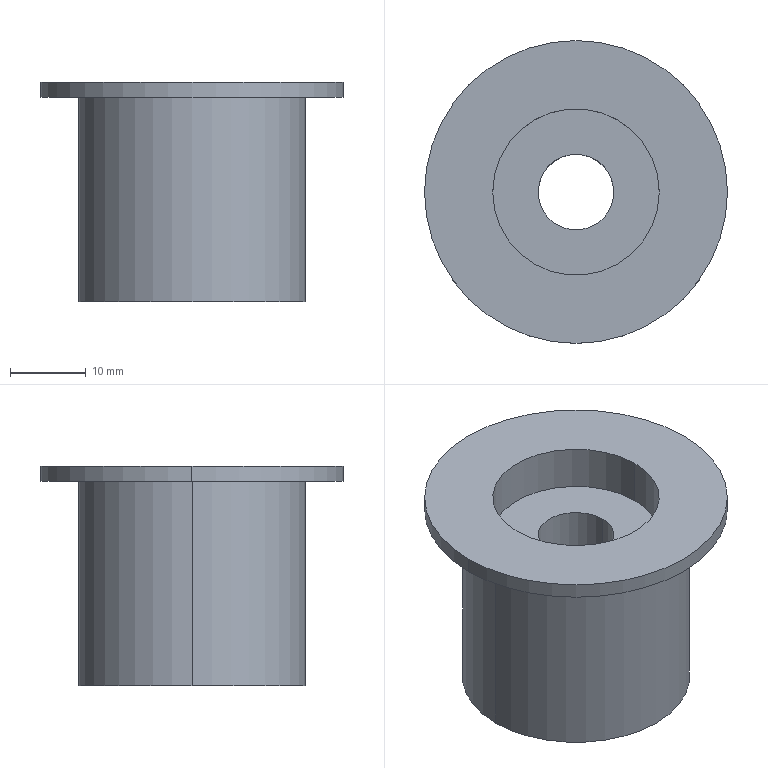Part | STEP file | Tensioning pulley QY-1-12 | 1 solid | 15 faces | box 40 x 40 x 29 mm | volume 15702 mm3 | cylinder 10 | plane 5 | commonest cylinder face diameters 22 x4 10 x2 30 x2 40 x2
STEP:
#1=CARTESIAN_POINT('',(0.,0.,0.));
#2=DIRECTION('',(0.,0.,1.));
#3=DIRECTION('',(1.,0.,0.));
#4=AXIS2_PLACEMENT_3D('',#1,#2,#3);
#5=CARTESIAN_POINT('',(20.,0.,12.5));
#6=VERTEX_POINT('',#5);
#7=CARTESIAN_POINT('',(-20.,0.,12.5));
#8=VERTEX_POINT('',#7);
#9=CARTESIAN_POINT('',(0.,0.,12.5));
#10=DIRECTION('',(0.,0.,1.));
#11=DIRECTION('',(1.,0.,0.));
#12=AXIS2_PLACEMENT_3D('',#9,#10,#11);
#13=CIRCLE('',#12,20.);
#14=CARTESIAN_POINT('',(0.,0.,12.5));
#15=DIRECTION('',(0.,0.,1.));
#16=DIRECTION('',(1.,0.,0.));
#17=AXIS2_PLACEMENT_3D('',#14,#15,#16);
#18=CYLINDRICAL_SURFACE('',#17,20.);
#19=CARTESIAN_POINT('',(0.,0.));
#20=DIRECTION('',(1.,0.));
#21=VECTOR('',#20,1.);
#22=LINE('',#19,#21);
#23=(GEOMETRIC_REPRESENTATION_CONTEXT(2)PARAMETRIC_REPRESENTATION_CONTEXT()REPRESENTATION_CONTEXT('',''));
#24=DEFINITIONAL_REPRESENTATION('',(#22),#23);
#25=PCURVE('',#18,#24);
#26=CARTESIAN_POINT('',(0.,0.,12.5));
#27=DIRECTION('',(0.,0.,1.));
#28=DIRECTION('',(1.,0.,0.));
#29=AXIS2_PLACEMENT_3D('',#26,#27,#28);
#30=PLANE('',#29);
#31=CARTESIAN_POINT('',(0.,0.));
#32=DIRECTION('',(1.,0.));
#33=AXIS2_PLACEMENT_2D('',#31,#32);
#34=CIRCLE('',#33,20.);
#35=(GEOMETRIC_REPRESENTATION_CONTEXT(2)PARAMETRIC_REPRESENTATION_CONTEXT()REPRESENTATION_CONTEXT('',''));
#36=DEFINITIONAL_REPRESENTATION('',(#34),#35);
#37=PCURVE('',#30,#36);
#38=SURFACE_CURVE('',#13,(#25,#37),.PCURVE_S1.);
#39=EDGE_CURVE('',#6,#8,#38,.T.);
#40=ORIENTED_EDGE('',*,*,#39,.T.);
#41=CARTESIAN_POINT('',(-20.,0.,14.5));
#42=VERTEX_POINT('',#41);
#43=CARTESIAN_POINT('',(-20.,0.,12.5));
#44=DIRECTION('',(0.,0.,1.));
#45=VECTOR('',#44,1.);
#46=LINE('',#43,#45);
#47=CARTESIAN_POINT('',(3.142,0.));
#48=DIRECTION('',(0.,1.));
#49=VECTOR('',#48,1.);
#50=LINE('',#47,#49);
#51=(GEOMETRIC_REPRESENTATION_CONTEXT(2)PARAMETRIC_REPRESENTATION_CONTEXT()REPRESENTATION_CONTEXT('',''));
#52=DEFINITIONAL_REPRESENTATION('',(#50),#51);
#53=PCURVE('',#18,#52);
#54=CARTESIAN_POINT('',(0.,0.,12.5));
#55=DIRECTION('',(0.,0.,1.));
#56=DIRECTION('',(1.,0.,0.));
#57=AXIS2_PLACEMENT_3D('',#54,#55,#56);
#58=CYLINDRICAL_SURFACE('',#57,20.);
#59=CARTESIAN_POINT('',(3.142,0.));
#60=DIRECTION('',(0.,1.));
#61=VECTOR('',#60,1.);
#62=LINE('',#59,#61);
#63=(GEOMETRIC_REPRESENTATION_CONTEXT(2)PARAMETRIC_REPRESENTATION_CONTEXT()REPRESENTATION_CONTEXT('',''));
#64=DEFINITIONAL_REPRESENTATION('',(#62),#63);
#65=PCURVE('',#58,#64);
#66=SURFACE_CURVE('',#46,(#53,#65),.PCURVE_S1.);
#67=EDGE_CURVE('',#8,#42,#66,.T.);
#68=ORIENTED_EDGE('',*,*,#67,.T.);
#69=CARTESIAN_POINT('',(20.,0.,14.5));
#70=VERTEX_POINT('',#69);
#71=CARTESIAN_POINT('',(0.,0.,14.5));
#72=DIRECTION('',(0.,0.,1.));
#73=DIRECTION('',(1.,0.,0.));
#74=AXIS2_PLACEMENT_3D('',#71,#72,#73);
#75=CIRCLE('',#74,20.);
#76=CARTESIAN_POINT('',(0.,2.));
#77=DIRECTION('',(1.,0.));
#78=VECTOR('',#77,1.);
#79=LINE('',#76,#78);
#80=(GEOMETRIC_REPRESENTATION_CONTEXT(2)PARAMETRIC_REPRESENTATION_CONTEXT()REPRESENTATION_CONTEXT('',''));
#81=DEFINITIONAL_REPRESENTATION('',(#79),#80);
#82=PCURVE('',#18,#81);
#83=CARTESIAN_POINT('',(0.,0.,14.5));
#84=DIRECTION('',(0.,0.,1.));
#85=DIRECTION('',(1.,0.,0.));
#86=AXIS2_PLACEMENT_3D('',#83,#84,#85);
#87=PLANE('',#86);
#88=CARTESIAN_POINT('',(0.,0.));
#89=DIRECTION('',(1.,0.));
#90=AXIS2_PLACEMENT_2D('',#88,#89);
#91=CIRCLE('',#90,20.);
#92=(GEOMETRIC_REPRESENTATION_CONTEXT(2)PARAMETRIC_REPRESENTATION_CONTEXT()REPRESENTATION_CONTEXT('',''));
#93=DEFINITIONAL_REPRESENTATION('',(#91),#92);
#94=PCURVE('',#87,#93);
#95=SURFACE_CURVE('',#75,(#82,#94),.PCURVE_S1.);
#96=EDGE_CURVE('',#70,#42,#95,.T.);
#97=ORIENTED_EDGE('',*,*,#96,.F.);
#98=CARTESIAN_POINT('',(20.,0.,12.5));
#99=DIRECTION('',(0.,0.,1.));
#100=VECTOR('',#99,1.);
#101=LINE('',#98,#100);
#102=CARTESIAN_POINT('',(0.,0.));
#103=DIRECTION('',(0.,1.));
#104=VECTOR('',#103,1.);
#105=LINE('',#102,#104);
#106=(GEOMETRIC_REPRESENTATION_CONTEXT(2)PARAMETRIC_REPRESENTATION_CONTEXT()REPRESENTATION_CONTEXT('',''));
#107=DEFINITIONAL_REPRESENTATION('',(#105),#106);
#108=PCURVE('',#18,#107);
#109=CARTESIAN_POINT('',(6.283,0.));
#110=DIRECTION('',(0.,1.));
#111=VECTOR('',#110,1.);
#112=LINE('',#109,#111);
#113=(GEOMETRIC_REPRESENTATION_CONTEXT(2)PARAMETRIC_REPRESENTATION_CONTEXT()REPRESENTATION_CONTEXT('',''));
#114=DEFINITIONAL_REPRESENTATION('',(#112),#113);
#115=PCURVE('',#58,#114);
#116=SURFACE_CURVE('',#101,(#108,#115),.PCURVE_S1.);
#117=EDGE_CURVE('',#6,#70,#116,.T.);
#118=ORIENTED_EDGE('',*,*,#117,.F.);
#119=EDGE_LOOP('',(#40,#68,#97,#118));
#120=FACE_BOUND('',#119,.T.);
#121=ADVANCED_FACE('',(#120),#18,.T.);
#122=CARTESIAN_POINT('',(-5.,0.,8.5));
#123=VERTEX_POINT('',#122);
#124=CARTESIAN_POINT('',(-5.,0.,-8.5));
#125=VERTEX_POINT('',#124);
#126=CARTESIAN_POINT('',(-5.,0.,8.5));
#127=DIRECTION('',(0.,0.,-1.));
#128=VECTOR('',#127,1.);
#129=LINE('',#126,#128);
#130=CARTESIAN_POINT('',(0.,0.,8.5));
#131=DIRECTION('',(0.,0.,-1.));
#132=DIRECTION('',(-1.,0.,0.));
#133=AXIS2_PLACEMENT_3D('',#130,#131,#132);
#134=CYLINDRICAL_SURFACE('',#133,5.);
#135=CARTESIAN_POINT('',(6.283,0.));
#136=DIRECTION('',(0.,1.));
#137=VECTOR('',#136,1.);
#138=LINE('',#135,#137);
#139=(GEOMETRIC_REPRESENTATION_CONTEXT(2)PARAMETRIC_REPRESENTATION_CONTEXT()REPRESENTATION_CONTEXT('',''));
#140=DEFINITIONAL_REPRESENTATION('',(#138),#139);
#141=PCURVE('',#134,#140);
#142=CARTESIAN_POINT('',(0.,0.,8.5));
#143=DIRECTION('',(0.,0.,-1.));
#144=DIRECTION('',(-1.,0.,0.));
#145=AXIS2_PLACEMENT_3D('',#142,#143,#144);
#146=CYLINDRICAL_SURFACE('',#145,5.);
#147=CARTESIAN_POINT('',(0.,0.));
#148=DIRECTION('',(0.,1.));
#149=VECTOR('',#148,1.);
#150=LINE('',#147,#149);
#151=(GEOMETRIC_REPRESENTATION_CONTEXT(2)PARAMETRIC_REPRESENTATION_CONTEXT()REPRESENTATION_CONTEXT('',''));
#152=DEFINITIONAL_REPRESENTATION('',(#150),#151);
#153=PCURVE('',#146,#152);
#154=SURFACE_CURVE('',#129,(#141,#153),.PCURVE_S1.);
#155=EDGE_CURVE('',#123,#125,#154,.T.);
#156=ORIENTED_EDGE('',*,*,#155,.T.);
#157=CARTESIAN_POINT('',(5.,0.,-8.5));
#158=VERTEX_POINT('',#157);
#159=CARTESIAN_POINT('',(0.,0.,-8.5));
#160=DIRECTION('',(0.,0.,1.));
#161=DIRECTION('',(1.,0.,0.));
#162=AXIS2_PLACEMENT_3D('',#159,#160,#161);
#163=CIRCLE('',#162,5.);
#164=CARTESIAN_POINT('',(9.425,17.));
#165=DIRECTION('',(-1.,0.));
#166=VECTOR('',#165,1.);
#167=LINE('',#164,#166);
#168=(GEOMETRIC_REPRESENTATION_CONTEXT(2)PARAMETRIC_REPRESENTATION_CONTEXT()REPRESENTATION_CONTEXT('',''));
#169=DEFINITIONAL_REPRESENTATION('',(#167),#168);
#170=PCURVE('',#134,#169);
#171=CARTESIAN_POINT('',(0.,0.,-8.5));
#172=DIRECTION('',(0.,0.,1.));
#173=DIRECTION('',(1.,0.,0.));
#174=AXIS2_PLACEMENT_3D('',#171,#172,#173);
#175=PLANE('',#174);
#176=CARTESIAN_POINT('',(0.,0.));
#177=DIRECTION('',(1.,0.));
#178=AXIS2_PLACEMENT_2D('',#176,#177);
#179=CIRCLE('',#178,5.);
#180=(GEOMETRIC_REPRESENTATION_CONTEXT(2)PARAMETRIC_REPRESENTATION_CONTEXT()REPRESENTATION_CONTEXT('',''));
#181=DEFINITIONAL_REPRESENTATION('',(#179),#180);
#182=PCURVE('',#175,#181);
#183=SURFACE_CURVE('',#163,(#170,#182),.PCURVE_S1.);
#184=EDGE_CURVE('',#125,#158,#183,.T.);
#185=ORIENTED_EDGE('',*,*,#184,.T.);
#186=CARTESIAN_POINT('',(5.,0.,8.5));
#187=VERTEX_POINT('',#186);
#188=CARTESIAN_POINT('',(5.,0.,8.5));
#189=DIRECTION('',(0.,0.,-1.));
#190=VECTOR('',#189,1.);
#191=LINE('',#188,#190);
#192=CARTESIAN_POINT('',(3.142,0.));
#193=DIRECTION('',(0.,1.));
#194=VECTOR('',#193,1.);
#195=LINE('',#192,#194);
#196=(GEOMETRIC_REPRESENTATION_CONTEXT(2)PARAMETRIC_REPRESENTATION_CONTEXT()REPRESENTATION_CONTEXT('',''));
#197=DEFINITIONAL_REPRESENTATION('',(#195),#196);
#198=PCURVE('',#134,#197);
#199=CARTESIAN_POINT('',(3.142,0.));
#200=DIRECTION('',(0.,1.));
#201=VECTOR('',#200,1.);
#202=LINE('',#199,#201);
#203=(GEOMETRIC_REPRESENTATION_CONTEXT(2)PARAMETRIC_REPRESENTATION_CONTEXT()REPRESENTATION_CONTEXT('',''));
#204=DEFINITIONAL_REPRESENTATION('',(#202),#203);
#205=PCURVE('',#146,#204);
#206=SURFACE_CURVE('',#191,(#198,#205),.PCURVE_S1.);
#207=EDGE_CURVE('',#187,#158,#206,.T.);
#208=ORIENTED_EDGE('',*,*,#207,.F.);
#209=CARTESIAN_POINT('',(0.,0.,8.5));
#210=DIRECTION('',(0.,0.,1.));
#211=DIRECTION('',(1.,0.,0.));
#212=AXIS2_PLACEMENT_3D('',#209,#210,#211);
#213=CIRCLE('',#212,5.);
#214=CARTESIAN_POINT('',(9.425,0.));
#215=DIRECTION('',(-1.,0.));
#216=VECTOR('',#215,1.);
#217=LINE('',#214,#216);
#218=(GEOMETRIC_REPRESENTATION_CONTEXT(2)PARAMETRIC_REPRESENTATION_CONTEXT()REPRESENTATION_CONTEXT('',''));
#219=DEFINITIONAL_REPRESENTATION('',(#217),#218);
#220=PCURVE('',#134,#219);
#221=CARTESIAN_POINT('',(0.,0.,8.5));
#222=DIRECTION('',(0.,0.,1.));
#223=DIRECTION('',(1.,0.,0.));
#224=AXIS2_PLACEMENT_3D('',#221,#222,#223);
#225=PLANE('',#224);
#226=CARTESIAN_POINT('',(0.,0.));
#227=DIRECTION('',(1.,0.));
#228=AXIS2_PLACEMENT_2D('',#226,#227);
#229=CIRCLE('',#228,5.);
#230=(GEOMETRIC_REPRESENTATION_CONTEXT(2)PARAMETRIC_REPRESENTATION_CONTEXT()REPRESENTATION_CONTEXT('',''));
#231=DEFINITIONAL_REPRESENTATION('',(#229),#230);
#232=PCURVE('',#225,#231);
#233=SURFACE_CURVE('',#213,(#220,#232),.PCURVE_S1.);
#234=EDGE_CURVE('',#123,#187,#233,.T.);
#235=ORIENTED_EDGE('',*,*,#234,.F.);
#236=EDGE_LOOP('',(#156,#185,#208,#235));
#237=FACE_BOUND('',#236,.F.);
#238=ADVANCED_FACE('',(#237),#134,.F.);
#239=CARTESIAN_POINT('',(-11.,0.,14.5));
#240=VERTEX_POINT('',#239);
#241=CARTESIAN_POINT('',(-11.,0.,8.5));
#242=VERTEX_POINT('',#241);
#243=CARTESIAN_POINT('',(-11.,0.,14.5));
#244=DIRECTION('',(0.,0.,-1.));
#245=VECTOR('',#244,1.);
#246=LINE('',#243,#245);
#247=CARTESIAN_POINT('',(0.,0.,14.5));
#248=DIRECTION('',(0.,0.,-1.));
#249=DIRECTION('',(-1.,0.,0.));
#250=AXIS2_PLACEMENT_3D('',#247,#248,#249);
#251=CYLINDRICAL_SURFACE('',#250,11.);
#252=CARTESIAN_POINT('',(6.283,0.));
#253=DIRECTION('',(0.,1.));
#254=VECTOR('',#253,1.);
#255=LINE('',#252,#254);
#256=(GEOMETRIC_REPRESENTATION_CONTEXT(2)PARAMETRIC_REPRESENTATION_CONTEXT()REPRESENTATION_CONTEXT('',''));
#257=DEFINITIONAL_REPRESENTATION('',(#255),#256);
#258=PCURVE('',#251,#257);
#259=CARTESIAN_POINT('',(0.,0.,14.5));
#260=DIRECTION('',(0.,0.,-1.));
#261=DIRECTION('',(-1.,0.,0.));
#262=AXIS2_PLACEMENT_3D('',#259,#260,#261);
#263=CYLINDRICAL_SURFACE('',#262,11.);
#264=CARTESIAN_POINT('',(0.,0.));
#265=DIRECTION('',(0.,1.));
#266=VECTOR('',#265,1.);
#267=LINE('',#264,#266);
#268=(GEOMETRIC_REPRESENTATION_CONTEXT(2)PARAMETRIC_REPRESENTATION_CONTEXT()REPRESENTATION_CONTEXT('',''));
#269=DEFINITIONAL_REPRESENTATION('',(#267),#268);
#270=PCURVE('',#263,#269);
#271=SURFACE_CURVE('',#246,(#258,#270),.PCURVE_S1.);
#272=EDGE_CURVE('',#240,#242,#271,.T.);
#273=ORIENTED_EDGE('',*,*,#272,.T.);
#274=CARTESIAN_POINT('',(11.,0.,8.5));
#275=VERTEX_POINT('',#274);
#276=CARTESIAN_POINT('',(0.,0.,8.5));
#277=DIRECTION('',(0.,0.,1.));
#278=DIRECTION('',(1.,0.,0.));
#279=AXIS2_PLACEMENT_3D('',#276,#277,#278);
#280=CIRCLE('',#279,11.);
#281=CARTESIAN_POINT('',(9.425,6.));
#282=DIRECTION('',(-1.,0.));
#283=VECTOR('',#282,1.);
#284=LINE('',#281,#283);
#285=(GEOMETRIC_REPRESENTATION_CONTEXT(2)PARAMETRIC_REPRESENTATION_CONTEXT()REPRESENTATION_CONTEXT('',''));
#286=DEFINITIONAL_REPRESENTATION('',(#284),#285);
#287=PCURVE('',#251,#286);
#288=CARTESIAN_POINT('',(0.,0.));
#289=DIRECTION('',(1.,0.));
#290=AXIS2_PLACEMENT_2D('',#288,#289);
#291=CIRCLE('',#290,11.);
#292=(GEOMETRIC_REPRESENTATION_CONTEXT(2)PARAMETRIC_REPRESENTATION_CONTEXT()REPRESENTATION_CONTEXT('',''));
#293=DEFINITIONAL_REPRESENTATION('',(#291),#292);
#294=PCURVE('',#225,#293);
#295=SURFACE_CURVE('',#280,(#287,#294),.PCURVE_S1.);
#296=EDGE_CURVE('',#242,#275,#295,.T.);
#297=ORIENTED_EDGE('',*,*,#296,.T.);
#298=CARTESIAN_POINT('',(11.,0.,14.5));
#299=VERTEX_POINT('',#298);
#300=CARTESIAN_POINT('',(11.,0.,14.5));
#301=DIRECTION('',(0.,0.,-1.));
#302=VECTOR('',#301,1.);
#303=LINE('',#300,#302);
#304=CARTESIAN_POINT('',(3.142,0.));
#305=DIRECTION('',(0.,1.));
#306=VECTOR('',#305,1.);
#307=LINE('',#304,#306);
#308=(GEOMETRIC_REPRESENTATION_CONTEXT(2)PARAMETRIC_REPRESENTATION_CONTEXT()REPRESENTATION_CONTEXT('',''));
#309=DEFINITIONAL_REPRESENTATION('',(#307),#308);
#310=PCURVE('',#251,#309);
#311=CARTESIAN_POINT('',(3.142,0.));
#312=DIRECTION('',(0.,1.));
#313=VECTOR('',#312,1.);
#314=LINE('',#311,#313);
#315=(GEOMETRIC_REPRESENTATION_CONTEXT(2)PARAMETRIC_REPRESENTATION_CONTEXT()REPRESENTATION_CONTEXT('',''));
#316=DEFINITIONAL_REPRESENTATION('',(#314),#315);
#317=PCURVE('',#263,#316);
#318=SURFACE_CURVE('',#303,(#310,#317),.PCURVE_S1.);
#319=EDGE_CURVE('',#299,#275,#318,.T.);
#320=ORIENTED_EDGE('',*,*,#319,.F.);
#321=CARTESIAN_POINT('',(0.,0.,14.5));
#322=DIRECTION('',(0.,0.,1.));
#323=DIRECTION('',(1.,0.,0.));
#324=AXIS2_PLACEMENT_3D('',#321,#322,#323);
#325=CIRCLE('',#324,11.);
#326=CARTESIAN_POINT('',(9.425,0.));
#327=DIRECTION('',(-1.,0.));
#328=VECTOR('',#327,1.);
#329=LINE('',#326,#328);
#330=(GEOMETRIC_REPRESENTATION_CONTEXT(2)PARAMETRIC_REPRESENTATION_CONTEXT()REPRESENTATION_CONTEXT('',''));
#331=DEFINITIONAL_REPRESENTATION('',(#329),#330);
#332=PCURVE('',#251,#331);
#333=CARTESIAN_POINT('',(0.,0.));
#334=DIRECTION('',(1.,0.));
#335=AXIS2_PLACEMENT_2D('',#333,#334);
#336=CIRCLE('',#335,11.);
#337=(GEOMETRIC_REPRESENTATION_CONTEXT(2)PARAMETRIC_REPRESENTATION_CONTEXT()REPRESENTATION_CONTEXT('',''));
#338=DEFINITIONAL_REPRESENTATION('',(#336),#337);
#339=PCURVE('',#87,#338);
#340=SURFACE_CURVE('',#325,(#332,#339),.PCURVE_S1.);
#341=EDGE_CURVE('',#240,#299,#340,.T.);
#342=ORIENTED_EDGE('',*,*,#341,.F.);
#343=EDGE_LOOP('',(#273,#297,#320,#342));
#344=FACE_BOUND('',#343,.F.);
#345=ADVANCED_FACE('',(#344),#251,.F.);
#346=CARTESIAN_POINT('',(-11.,0.,-8.5));
#347=VERTEX_POINT('',#346);
#348=CARTESIAN_POINT('',(-11.,0.,-14.5));
#349=VERTEX_POINT('',#348);
#350=CARTESIAN_POINT('',(-11.,0.,14.5));
#351=DIRECTION('',(0.,0.,-1.));
#352=VECTOR('',#351,1.);
#353=LINE('',#350,#352);
#354=CARTESIAN_POINT('',(0.,0.,14.5));
#355=DIRECTION('',(0.,0.,-1.));
#356=DIRECTION('',(-1.,0.,0.));
#357=AXIS2_PLACEMENT_3D('',#354,#355,#356);
#358=CYLINDRICAL_SURFACE('',#357,11.);
#359=CARTESIAN_POINT('',(6.283,0.));
#360=DIRECTION('',(0.,1.));
#361=VECTOR('',#360,1.);
#362=LINE('',#359,#361);
#363=(GEOMETRIC_REPRESENTATION_CONTEXT(2)PARAMETRIC_REPRESENTATION_CONTEXT()REPRESENTATION_CONTEXT('',''));
#364=DEFINITIONAL_REPRESENTATION('',(#362),#363);
#365=PCURVE('',#358,#364);
#366=CARTESIAN_POINT('',(0.,0.,14.5));
#367=DIRECTION('',(0.,0.,-1.));
#368=DIRECTION('',(-1.,0.,0.));
#369=AXIS2_PLACEMENT_3D('',#366,#367,#368);
#370=CYLINDRICAL_SURFACE('',#369,11.);
#371=CARTESIAN_POINT('',(0.,0.));
#372=DIRECTION('',(0.,1.));
#373=VECTOR('',#372,1.);
#374=LINE('',#371,#373);
#375=(GEOMETRIC_REPRESENTATION_CONTEXT(2)PARAMETRIC_REPRESENTATION_CONTEXT()REPRESENTATION_CONTEXT('',''));
#376=DEFINITIONAL_REPRESENTATION('',(#374),#375);
#377=PCURVE('',#370,#376);
#378=SURFACE_CURVE('',#353,(#365,#377),.PCURVE_S1.);
#379=EDGE_CURVE('',#347,#349,#378,.T.);
#380=ORIENTED_EDGE('',*,*,#379,.T.);
#381=CARTESIAN_POINT('',(11.,0.,-14.5));
#382=VERTEX_POINT('',#381);
#383=CARTESIAN_POINT('',(0.,0.,-14.5));
#384=DIRECTION('',(0.,0.,1.));
#385=DIRECTION('',(1.,0.,0.));
#386=AXIS2_PLACEMENT_3D('',#383,#384,#385);
#387=CIRCLE('',#386,11.);
#388=CARTESIAN_POINT('',(9.425,29.));
#389=DIRECTION('',(-1.,0.));
#390=VECTOR('',#389,1.);
#391=LINE('',#388,#390);
#392=(GEOMETRIC_REPRESENTATION_CONTEXT(2)PARAMETRIC_REPRESENTATION_CONTEXT()REPRESENTATION_CONTEXT('',''));
#393=DEFINITIONAL_REPRESENTATION('',(#391),#392);
#394=PCURVE('',#358,#393);
#395=CARTESIAN_POINT('',(0.,0.,-14.5));
#396=DIRECTION('',(0.,0.,1.));
#397=DIRECTION('',(1.,0.,0.));
#398=AXIS2_PLACEMENT_3D('',#395,#396,#397);
#399=PLANE('',#398);
#400=CARTESIAN_POINT('',(0.,0.));
#401=DIRECTION('',(1.,0.));
#402=AXIS2_PLACEMENT_2D('',#400,#401);
#403=CIRCLE('',#402,11.);
#404=(GEOMETRIC_REPRESENTATION_CONTEXT(2)PARAMETRIC_REPRESENTATION_CONTEXT()REPRESENTATION_CONTEXT('',''));
#405=DEFINITIONAL_REPRESENTATION('',(#403),#404);
#406=PCURVE('',#399,#405);
#407=SURFACE_CURVE('',#387,(#394,#406),.PCURVE_S1.);
#408=EDGE_CURVE('',#349,#382,#407,.T.);
#409=ORIENTED_EDGE('',*,*,#408,.T.);
#410=CARTESIAN_POINT('',(11.,0.,-8.5));
#411=VERTEX_POINT('',#410);
#412=CARTESIAN_POINT('',(11.,0.,14.5));
#413=DIRECTION('',(0.,0.,-1.));
#414=VECTOR('',#413,1.);
#415=LINE('',#412,#414);
#416=CARTESIAN_POINT('',(3.142,0.));
#417=DIRECTION('',(0.,1.));
#418=VECTOR('',#417,1.);
#419=LINE('',#416,#418);
#420=(GEOMETRIC_REPRESENTATION_CONTEXT(2)PARAMETRIC_REPRESENTATION_CONTEXT()REPRESENTATION_CONTEXT('',''));
#421=DEFINITIONAL_REPRESENTATION('',(#419),#420);
#422=PCURVE('',#358,#421);
#423=CARTESIAN_POINT('',(3.142,0.));
#424=DIRECTION('',(0.,1.));
#425=VECTOR('',#424,1.);
#426=LINE('',#423,#425);
#427=(GEOMETRIC_REPRESENTATION_CONTEXT(2)PARAMETRIC_REPRESENTATION_CONTEXT()REPRESENTATION_CONTEXT('',''));
#428=DEFINITIONAL_REPRESENTATION('',(#426),#427);
#429=PCURVE('',#370,#428);
#430=SURFACE_CURVE('',#415,(#422,#429),.PCURVE_S1.);
#431=EDGE_CURVE('',#411,#382,#430,.T.);
#432=ORIENTED_EDGE('',*,*,#431,.F.);
#433=CARTESIAN_POINT('',(0.,0.,-8.5));
#434=DIRECTION('',(0.,0.,1.));
#435=DIRECTION('',(1.,0.,0.));
#436=AXIS2_PLACEMENT_3D('',#433,#434,#435);
#437=CIRCLE('',#436,11.);
#438=CARTESIAN_POINT('',(9.425,23.));
#439=DIRECTION('',(-1.,0.));
#440=VECTOR('',#439,1.);
#441=LINE('',#438,#440);
#442=(GEOMETRIC_REPRESENTATION_CONTEXT(2)PARAMETRIC_REPRESENTATION_CONTEXT()REPRESENTATION_CONTEXT('',''));
#443=DEFINITIONAL_REPRESENTATION('',(#441),#442);
#444=PCURVE('',#358,#443);
#445=CARTESIAN_POINT('',(0.,0.));
#446=DIRECTION('',(1.,0.));
#447=AXIS2_PLACEMENT_2D('',#445,#446);
#448=CIRCLE('',#447,11.);
#449=(GEOMETRIC_REPRESENTATION_CONTEXT(2)PARAMETRIC_REPRESENTATION_CONTEXT()REPRESENTATION_CONTEXT('',''));
#450=DEFINITIONAL_REPRESENTATION('',(#448),#449);
#451=PCURVE('',#175,#450);
#452=SURFACE_CURVE('',#437,(#444,#451),.PCURVE_S1.);
#453=EDGE_CURVE('',#347,#411,#452,.T.);
#454=ORIENTED_EDGE('',*,*,#453,.F.);
#455=EDGE_LOOP('',(#380,#409,#432,#454));
#456=FACE_BOUND('',#455,.F.);
#457=ADVANCED_FACE('',(#456),#358,.F.);
#458=CARTESIAN_POINT('',(15.,0.,12.5));
#459=VERTEX_POINT('',#458);
#460=CARTESIAN_POINT('',(-15.,0.,12.5));
#461=VERTEX_POINT('',#460);
#462=CARTESIAN_POINT('',(0.,0.,12.5));
#463=DIRECTION('',(0.,0.,1.));
#464=DIRECTION('',(1.,0.,0.));
#465=AXIS2_PLACEMENT_3D('',#462,#463,#464);
#466=CIRCLE('',#465,15.);
#467=CARTESIAN_POINT('',(0.,0.,14.5));
#468=DIRECTION('',(0.,0.,-1.));
#469=DIRECTION('',(-1.,0.,0.));
#470=AXIS2_PLACEMENT_3D('',#467,#468,#469);
#471=CYLINDRICAL_SURFACE('',#470,15.);
#472=CARTESIAN_POINT('',(3.142,2.));
#473=DIRECTION('',(-1.,0.));
#474=VECTOR('',#473,1.);
#475=LINE('',#472,#474);
#476=(GEOMETRIC_REPRESENTATION_CONTEXT(2)PARAMETRIC_REPRESENTATION_CONTEXT()REPRESENTATION_CONTEXT('',''));
#477=DEFINITIONAL_REPRESENTATION('',(#475),#476);
#478=PCURVE('',#471,#477);
#479=CARTESIAN_POINT('',(0.,0.));
#480=DIRECTION('',(1.,0.));
#481=AXIS2_PLACEMENT_2D('',#479,#480);
#482=CIRCLE('',#481,15.);
#483=(GEOMETRIC_REPRESENTATION_CONTEXT(2)PARAMETRIC_REPRESENTATION_CONTEXT()REPRESENTATION_CONTEXT('',''));
#484=DEFINITIONAL_REPRESENTATION('',(#482),#483);
#485=PCURVE('',#30,#484);
#486=SURFACE_CURVE('',#466,(#478,#485),.PCURVE_S1.);
#487=EDGE_CURVE('',#459,#461,#486,.T.);
#488=ORIENTED_EDGE('',*,*,#487,.F.);
#489=CARTESIAN_POINT('',(15.,0.,-14.5));
#490=VERTEX_POINT('',#489);
#491=CARTESIAN_POINT('',(15.,0.,14.5));
#492=DIRECTION('',(0.,0.,-1.));
#493=VECTOR('',#492,1.);
#494=LINE('',#491,#493);
#495=CARTESIAN_POINT('',(3.142,0.));
#496=DIRECTION('',(0.,1.));
#497=VECTOR('',#496,1.);
#498=LINE('',#495,#497);
#499=(GEOMETRIC_REPRESENTATION_CONTEXT(2)PARAMETRIC_REPRESENTATION_CONTEXT()REPRESENTATION_CONTEXT('',''));
#500=DEFINITIONAL_REPRESENTATION('',(#498),#499);
#501=PCURVE('',#471,#500);
#502=CARTESIAN_POINT('',(0.,0.,14.5));
#503=DIRECTION('',(0.,0.,-1.));
#504=DIRECTION('',(-1.,0.,0.));
#505=AXIS2_PLACEMENT_3D('',#502,#503,#504);
#506=CYLINDRICAL_SURFACE('',#505,15.);
#507=CARTESIAN_POINT('',(3.142,0.));
#508=DIRECTION('',(0.,1.));
#509=VECTOR('',#508,1.);
#510=LINE('',#507,#509);
#511=(GEOMETRIC_REPRESENTATION_CONTEXT(2)PARAMETRIC_REPRESENTATION_CONTEXT()REPRESENTATION_CONTEXT('',''));
#512=DEFINITIONAL_REPRESENTATION('',(#510),#511);
#513=PCURVE('',#506,#512);
#514=SURFACE_CURVE('',#494,(#501,#513),.PCURVE_S1.);
#515=EDGE_CURVE('',#459,#490,#514,.T.);
#516=ORIENTED_EDGE('',*,*,#515,.T.);
#517=CARTESIAN_POINT('',(-15.,0.,-14.5));
#518=VERTEX_POINT('',#517);
#519=CARTESIAN_POINT('',(0.,0.,-14.5));
#520=DIRECTION('',(0.,0.,1.));
#521=DIRECTION('',(1.,0.,0.));
#522=AXIS2_PLACEMENT_3D('',#519,#520,#521);
#523=CIRCLE('',#522,15.);
#524=CARTESIAN_POINT('',(3.142,29.));
#525=DIRECTION('',(-1.,0.));
#526=VECTOR('',#525,1.);
#527=LINE('',#524,#526);
#528=(GEOMETRIC_REPRESENTATION_CONTEXT(2)PARAMETRIC_REPRESENTATION_CONTEXT()REPRESENTATION_CONTEXT('',''));
#529=DEFINITIONAL_REPRESENTATION('',(#527),#528);
#530=PCURVE('',#471,#529);
#531=CARTESIAN_POINT('',(0.,0.));
#532=DIRECTION('',(1.,0.));
#533=AXIS2_PLACEMENT_2D('',#531,#532);
#534=CIRCLE('',#533,15.);
#535=(GEOMETRIC_REPRESENTATION_CONTEXT(2)PARAMETRIC_REPRESENTATION_CONTEXT()REPRESENTATION_CONTEXT('',''));
#536=DEFINITIONAL_REPRESENTATION('',(#534),#535);
#537=PCURVE('',#399,#536);
#538=SURFACE_CURVE('',#523,(#530,#537),.PCURVE_S1.);
#539=EDGE_CURVE('',#490,#518,#538,.T.);
#540=ORIENTED_EDGE('',*,*,#539,.T.);
#541=CARTESIAN_POINT('',(-15.,0.,14.5));
#542=DIRECTION('',(0.,0.,-1.));
#543=VECTOR('',#542,1.);
#544=LINE('',#541,#543);
#545=CARTESIAN_POINT('',(0.,0.));
#546=DIRECTION('',(0.,1.));
#547=VECTOR('',#546,1.);
#548=LINE('',#545,#547);
#549=(GEOMETRIC_REPRESENTATION_CONTEXT(2)PARAMETRIC_REPRESENTATION_CONTEXT()REPRESENTATION_CONTEXT('',''));
#550=DEFINITIONAL_REPRESENTATION('',(#548),#549);
#551=PCURVE('',#471,#550);
#552=CARTESIAN_POINT('',(6.283,0.));
#553=DIRECTION('',(0.,1.));
#554=VECTOR('',#553,1.);
#555=LINE('',#552,#554);
#556=(GEOMETRIC_REPRESENTATION_CONTEXT(2)PARAMETRIC_REPRESENTATION_CONTEXT()REPRESENTATION_CONTEXT('',''));
#557=DEFINITIONAL_REPRESENTATION('',(#555),#556);
#558=PCURVE('',#506,#557);
#559=SURFACE_CURVE('',#544,(#551,#558),.PCURVE_S1.);
#560=EDGE_CURVE('',#461,#518,#559,.T.);
#561=ORIENTED_EDGE('',*,*,#560,.F.);
#562=EDGE_LOOP('',(#488,#516,#540,#561));
#563=FACE_BOUND('',#562,.T.);
#564=ADVANCED_FACE('',(#563),#471,.T.);
#565=ORIENTED_EDGE('',*,*,#515,.F.);
#566=CARTESIAN_POINT('',(0.,0.,12.5));
#567=DIRECTION('',(0.,0.,1.));
#568=DIRECTION('',(1.,0.,0.));
#569=AXIS2_PLACEMENT_3D('',#566,#567,#568);
#570=CIRCLE('',#569,15.);
#571=CARTESIAN_POINT('',(9.425,2.));
#572=DIRECTION('',(-1.,0.));
#573=VECTOR('',#572,1.);
#574=LINE('',#571,#573);
#575=(GEOMETRIC_REPRESENTATION_CONTEXT(2)PARAMETRIC_REPRESENTATION_CONTEXT()REPRESENTATION_CONTEXT('',''));
#576=DEFINITIONAL_REPRESENTATION('',(#574),#575);
#577=PCURVE('',#506,#576);
#578=CARTESIAN_POINT('',(0.,0.));
#579=DIRECTION('',(1.,0.));
#580=AXIS2_PLACEMENT_2D('',#578,#579);
#581=CIRCLE('',#580,15.);
#582=(GEOMETRIC_REPRESENTATION_CONTEXT(2)PARAMETRIC_REPRESENTATION_CONTEXT()REPRESENTATION_CONTEXT('',''));
#583=DEFINITIONAL_REPRESENTATION('',(#581),#582);
#584=PCURVE('',#30,#583);
#585=SURFACE_CURVE('',#570,(#577,#584),.PCURVE_S1.);
#586=EDGE_CURVE('',#461,#459,#585,.T.);
#587=ORIENTED_EDGE('',*,*,#586,.F.);
#588=ORIENTED_EDGE('',*,*,#560,.T.);
#589=CARTESIAN_POINT('',(0.,0.,-14.5));
#590=DIRECTION('',(0.,0.,1.));
#591=DIRECTION('',(1.,0.,0.));
#592=AXIS2_PLACEMENT_3D('',#589,#590,#591);
#593=CIRCLE('',#592,15.);
#594=CARTESIAN_POINT('',(9.425,29.));
#595=DIRECTION('',(-1.,0.));
#596=VECTOR('',#595,1.);
#597=LINE('',#594,#596);
#598=(GEOMETRIC_REPRESENTATION_CONTEXT(2)PARAMETRIC_REPRESENTATION_CONTEXT()REPRESENTATION_CONTEXT('',''));
#599=DEFINITIONAL_REPRESENTATION('',(#597),#598);
#600=PCURVE('',#506,#599);
#601=CARTESIAN_POINT('',(0.,0.));
#602=DIRECTION('',(1.,0.));
#603=AXIS2_PLACEMENT_2D('',#601,#602);
#604=CIRCLE('',#603,15.);
#605=(GEOMETRIC_REPRESENTATION_CONTEXT(2)PARAMETRIC_REPRESENTATION_CONTEXT()REPRESENTATION_CONTEXT('',''));
#606=DEFINITIONAL_REPRESENTATION('',(#604),#605);
#607=PCURVE('',#399,#606);
#608=SURFACE_CURVE('',#593,(#600,#607),.PCURVE_S1.);
#609=EDGE_CURVE('',#518,#490,#608,.T.);
#610=ORIENTED_EDGE('',*,*,#609,.T.);
#611=EDGE_LOOP('',(#565,#587,#588,#610));
#612=FACE_BOUND('',#611,.T.);
#613=ADVANCED_FACE('',(#612),#506,.T.);
#614=CARTESIAN_POINT('',(0.,0.,-14.5));
#615=DIRECTION('',(0.,0.,1.));
#616=DIRECTION('',(1.,0.,0.));
#617=AXIS2_PLACEMENT_3D('',#614,#615,#616);
#618=CIRCLE('',#617,11.);
#619=CARTESIAN_POINT('',(3.142,29.));
#620=DIRECTION('',(-1.,0.));
#621=VECTOR('',#620,1.);
#622=LINE('',#619,#621);
#623=(GEOMETRIC_REPRESENTATION_CONTEXT(2)PARAMETRIC_REPRESENTATION_CONTEXT()REPRESENTATION_CONTEXT('',''));
#624=DEFINITIONAL_REPRESENTATION('',(#622),#623);
#625=PCURVE('',#370,#624);
#626=CARTESIAN_POINT('',(0.,0.));
#627=DIRECTION('',(1.,0.));
#628=AXIS2_PLACEMENT_2D('',#626,#627);
#629=CIRCLE('',#628,11.);
#630=(GEOMETRIC_REPRESENTATION_CONTEXT(2)PARAMETRIC_REPRESENTATION_CONTEXT()REPRESENTATION_CONTEXT('',''));
#631=DEFINITIONAL_REPRESENTATION('',(#629),#630);
#632=PCURVE('',#399,#631);
#633=SURFACE_CURVE('',#618,(#625,#632),.PCURVE_S1.);
#634=EDGE_CURVE('',#382,#349,#633,.T.);
#635=ORIENTED_EDGE('',*,*,#634,.T.);
#636=ORIENTED_EDGE('',*,*,#379,.F.);
#637=CARTESIAN_POINT('',(0.,0.,-8.5));
#638=DIRECTION('',(0.,0.,1.));
#639=DIRECTION('',(1.,0.,0.));
#640=AXIS2_PLACEMENT_3D('',#637,#638,#639);
#641=CIRCLE('',#640,11.);
#642=CARTESIAN_POINT('',(3.142,23.));
#643=DIRECTION('',(-1.,0.));
#644=VECTOR('',#643,1.);
#645=LINE('',#642,#644);
#646=(GEOMETRIC_REPRESENTATION_CONTEXT(2)PARAMETRIC_REPRESENTATION_CONTEXT()REPRESENTATION_CONTEXT('',''));
#647=DEFINITIONAL_REPRESENTATION('',(#645),#646);
#648=PCURVE('',#370,#647);
#649=CARTESIAN_POINT('',(0.,0.));
#650=DIRECTION('',(1.,0.));
#651=AXIS2_PLACEMENT_2D('',#649,#650);
#652=CIRCLE('',#651,11.);
#653=(GEOMETRIC_REPRESENTATION_CONTEXT(2)PARAMETRIC_REPRESENTATION_CONTEXT()REPRESENTATION_CONTEXT('',''));
#654=DEFINITIONAL_REPRESENTATION('',(#652),#653);
#655=PCURVE('',#175,#654);
#656=SURFACE_CURVE('',#641,(#648,#655),.PCURVE_S1.);
#657=EDGE_CURVE('',#411,#347,#656,.T.);
#658=ORIENTED_EDGE('',*,*,#657,.F.);
#659=ORIENTED_EDGE('',*,*,#431,.T.);
#660=EDGE_LOOP('',(#635,#636,#658,#659));
#661=FACE_BOUND('',#660,.F.);
#662=ADVANCED_FACE('',(#661),#370,.F.);
#663=ORIENTED_EDGE('',*,*,#341,.F.);
#664=CARTESIAN_POINT('',(0.,0.,14.5));
#665=DIRECTION('',(0.,0.,1.));
#666=DIRECTION('',(1.,0.,0.));
#667=AXIS2_PLACEMENT_3D('',#664,#665,#666);
#668=CIRCLE('',#667,11.);
#669=CARTESIAN_POINT('',(0.,0.));
#670=DIRECTION('',(1.,0.));
#671=AXIS2_PLACEMENT_2D('',#669,#670);
#672=CIRCLE('',#671,11.);
#673=(GEOMETRIC_REPRESENTATION_CONTEXT(2)PARAMETRIC_REPRESENTATION_CONTEXT()REPRESENTATION_CONTEXT('',''));
#674=DEFINITIONAL_REPRESENTATION('',(#672),#673);
#675=PCURVE('',#87,#674);
#676=CARTESIAN_POINT('',(3.142,0.));
#677=DIRECTION('',(-1.,0.));
#678=VECTOR('',#677,1.);
#679=LINE('',#676,#678);
#680=(GEOMETRIC_REPRESENTATION_CONTEXT(2)PARAMETRIC_REPRESENTATION_CONTEXT()REPRESENTATION_CONTEXT('',''));
#681=DEFINITIONAL_REPRESENTATION('',(#679),#680);
#682=PCURVE('',#263,#681);
#683=SURFACE_CURVE('',#668,(#675,#682),.PCURVE_S1.);
#684=EDGE_CURVE('',#299,#240,#683,.T.);
#685=ORIENTED_EDGE('',*,*,#684,.F.);
#686=EDGE_LOOP('',(#663,#685));
#687=FACE_BOUND('',#686,.T.);
#688=ORIENTED_EDGE('',*,*,#96,.T.);
#689=CARTESIAN_POINT('',(0.,0.,14.5));
#690=DIRECTION('',(0.,0.,1.));
#691=DIRECTION('',(1.,0.,0.));
#692=AXIS2_PLACEMENT_3D('',#689,#690,#691);
#693=CIRCLE('',#692,20.);
#694=CARTESIAN_POINT('',(0.,0.));
#695=DIRECTION('',(1.,0.));
#696=AXIS2_PLACEMENT_2D('',#694,#695);
#697=CIRCLE('',#696,20.);
#698=(GEOMETRIC_REPRESENTATION_CONTEXT(2)PARAMETRIC_REPRESENTATION_CONTEXT()REPRESENTATION_CONTEXT('',''));
#699=DEFINITIONAL_REPRESENTATION('',(#697),#698);
#700=PCURVE('',#87,#699);
#701=CARTESIAN_POINT('',(0.,2.));
#702=DIRECTION('',(1.,0.));
#703=VECTOR('',#702,1.);
#704=LINE('',#701,#703);
#705=(GEOMETRIC_REPRESENTATION_CONTEXT(2)PARAMETRIC_REPRESENTATION_CONTEXT()REPRESENTATION_CONTEXT('',''));
#706=DEFINITIONAL_REPRESENTATION('',(#704),#705);
#707=PCURVE('',#58,#706);
#708=SURFACE_CURVE('',#693,(#700,#707),.PCURVE_S1.);
#709=EDGE_CURVE('',#42,#70,#708,.T.);
#710=ORIENTED_EDGE('',*,*,#709,.T.);
#711=EDGE_LOOP('',(#688,#710));
#712=FACE_BOUND('',#711,.T.);
#713=ADVANCED_FACE('',(#687,#712),#87,.T.);
#714=ORIENTED_EDGE('',*,*,#609,.F.);
#715=ORIENTED_EDGE('',*,*,#539,.F.);
#716=EDGE_LOOP('',(#714,#715));
#717=FACE_BOUND('',#716,.T.);
#718=ORIENTED_EDGE('',*,*,#408,.T.);
#719=ORIENTED_EDGE('',*,*,#634,.T.);
#720=EDGE_LOOP('',(#718,#719));
#721=FACE_BOUND('',#720,.T.);
#722=ADVANCED_FACE('',(#717,#721),#399,.F.);
#723=CARTESIAN_POINT('',(0.,0.,8.5));
#724=DIRECTION('',(0.,0.,1.));
#725=DIRECTION('',(1.,0.,0.));
#726=AXIS2_PLACEMENT_3D('',#723,#724,#725);
#727=CIRCLE('',#726,11.);
#728=CARTESIAN_POINT('',(3.142,6.));
#729=DIRECTION('',(-1.,0.));
#730=VECTOR('',#729,1.);
#731=LINE('',#728,#730);
#732=(GEOMETRIC_REPRESENTATION_CONTEXT(2)PARAMETRIC_REPRESENTATION_CONTEXT()REPRESENTATION_CONTEXT('',''));
#733=DEFINITIONAL_REPRESENTATION('',(#731),#732);
#734=PCURVE('',#263,#733);
#735=CARTESIAN_POINT('',(0.,0.));
#736=DIRECTION('',(1.,0.));
#737=AXIS2_PLACEMENT_2D('',#735,#736);
#738=CIRCLE('',#737,11.);
#739=(GEOMETRIC_REPRESENTATION_CONTEXT(2)PARAMETRIC_REPRESENTATION_CONTEXT()REPRESENTATION_CONTEXT('',''));
#740=DEFINITIONAL_REPRESENTATION('',(#738),#739);
#741=PCURVE('',#225,#740);
#742=SURFACE_CURVE('',#727,(#734,#741),.PCURVE_S1.);
#743=EDGE_CURVE('',#275,#242,#742,.T.);
#744=ORIENTED_EDGE('',*,*,#743,.T.);
#745=ORIENTED_EDGE('',*,*,#272,.F.);
#746=ORIENTED_EDGE('',*,*,#684,.F.);
#747=ORIENTED_EDGE('',*,*,#319,.T.);
#748=EDGE_LOOP('',(#744,#745,#746,#747));
#749=FACE_BOUND('',#748,.F.);
#750=ADVANCED_FACE('',(#749),#263,.F.);
#751=ORIENTED_EDGE('',*,*,#234,.F.);
#752=CARTESIAN_POINT('',(0.,0.,8.5));
#753=DIRECTION('',(0.,0.,1.));
#754=DIRECTION('',(1.,0.,0.));
#755=AXIS2_PLACEMENT_3D('',#752,#753,#754);
#756=CIRCLE('',#755,5.);
#757=CARTESIAN_POINT('',(0.,0.));
#758=DIRECTION('',(1.,0.));
#759=AXIS2_PLACEMENT_2D('',#757,#758);
#760=CIRCLE('',#759,5.);
#761=(GEOMETRIC_REPRESENTATION_CONTEXT(2)PARAMETRIC_REPRESENTATION_CONTEXT()REPRESENTATION_CONTEXT('',''));
#762=DEFINITIONAL_REPRESENTATION('',(#760),#761);
#763=PCURVE('',#225,#762);
#764=CARTESIAN_POINT('',(3.142,0.));
#765=DIRECTION('',(-1.,0.));
#766=VECTOR('',#765,1.);
#767=LINE('',#764,#766);
#768=(GEOMETRIC_REPRESENTATION_CONTEXT(2)PARAMETRIC_REPRESENTATION_CONTEXT()REPRESENTATION_CONTEXT('',''));
#769=DEFINITIONAL_REPRESENTATION('',(#767),#768);
#770=PCURVE('',#146,#769);
#771=SURFACE_CURVE('',#756,(#763,#770),.PCURVE_S1.);
#772=EDGE_CURVE('',#187,#123,#771,.T.);
#773=ORIENTED_EDGE('',*,*,#772,.F.);
#774=EDGE_LOOP('',(#751,#773));
#775=FACE_BOUND('',#774,.T.);
#776=ORIENTED_EDGE('',*,*,#296,.T.);
#777=ORIENTED_EDGE('',*,*,#743,.T.);
#778=EDGE_LOOP('',(#776,#777));
#779=FACE_BOUND('',#778,.T.);
#780=ADVANCED_FACE('',(#775,#779),#225,.T.);
#781=ORIENTED_EDGE('',*,*,#184,.T.);
#782=CARTESIAN_POINT('',(0.,0.,-8.5));
#783=DIRECTION('',(0.,0.,1.));
#784=DIRECTION('',(1.,0.,0.));
#785=AXIS2_PLACEMENT_3D('',#782,#783,#784);
#786=CIRCLE('',#785,5.);
#787=CARTESIAN_POINT('',(0.,0.));
#788=DIRECTION('',(1.,0.));
#789=AXIS2_PLACEMENT_2D('',#787,#788);
#790=CIRCLE('',#789,5.);
#791=(GEOMETRIC_REPRESENTATION_CONTEXT(2)PARAMETRIC_REPRESENTATION_CONTEXT()REPRESENTATION_CONTEXT('',''));
#792=DEFINITIONAL_REPRESENTATION('',(#790),#791);
#793=PCURVE('',#175,#792);
#794=CARTESIAN_POINT('',(3.142,17.));
#795=DIRECTION('',(-1.,0.));
#796=VECTOR('',#795,1.);
#797=LINE('',#794,#796);
#798=(GEOMETRIC_REPRESENTATION_CONTEXT(2)PARAMETRIC_REPRESENTATION_CONTEXT()REPRESENTATION_CONTEXT('',''));
#799=DEFINITIONAL_REPRESENTATION('',(#797),#798);
#800=PCURVE('',#146,#799);
#801=SURFACE_CURVE('',#786,(#793,#800),.PCURVE_S1.);
#802=EDGE_CURVE('',#158,#125,#801,.T.);
#803=ORIENTED_EDGE('',*,*,#802,.T.);
#804=EDGE_LOOP('',(#781,#803));
#805=FACE_BOUND('',#804,.T.);
#806=ORIENTED_EDGE('',*,*,#453,.F.);
#807=ORIENTED_EDGE('',*,*,#657,.F.);
#808=EDGE_LOOP('',(#806,#807));
#809=FACE_BOUND('',#808,.T.);
#810=ADVANCED_FACE('',(#805,#809),#175,.F.);
#811=ORIENTED_EDGE('',*,*,#802,.T.);
#812=ORIENTED_EDGE('',*,*,#155,.F.);
#813=ORIENTED_EDGE('',*,*,#772,.F.);
#814=ORIENTED_EDGE('',*,*,#207,.T.);
#815=EDGE_LOOP('',(#811,#812,#813,#814));
#816=FACE_BOUND('',#815,.F.);
#817=ADVANCED_FACE('',(#816),#146,.F.);
#818=ORIENTED_EDGE('',*,*,#67,.F.);
#819=CARTESIAN_POINT('',(0.,0.,12.5));
#820=DIRECTION('',(0.,0.,1.));
#821=DIRECTION('',(1.,0.,0.));
#822=AXIS2_PLACEMENT_3D('',#819,#820,#821);
#823=CIRCLE('',#822,20.);
#824=CARTESIAN_POINT('',(0.,0.));
#825=DIRECTION('',(1.,0.));
#826=VECTOR('',#825,1.);
#827=LINE('',#824,#826);
#828=(GEOMETRIC_REPRESENTATION_CONTEXT(2)PARAMETRIC_REPRESENTATION_CONTEXT()REPRESENTATION_CONTEXT('',''));
#829=DEFINITIONAL_REPRESENTATION('',(#827),#828);
#830=PCURVE('',#58,#829);
#831=CARTESIAN_POINT('',(0.,0.));
#832=DIRECTION('',(1.,0.));
#833=AXIS2_PLACEMENT_2D('',#831,#832);
#834=CIRCLE('',#833,20.);
#835=(GEOMETRIC_REPRESENTATION_CONTEXT(2)PARAMETRIC_REPRESENTATION_CONTEXT()REPRESENTATION_CONTEXT('',''));
#836=DEFINITIONAL_REPRESENTATION('',(#834),#835);
#837=PCURVE('',#30,#836);
#838=SURFACE_CURVE('',#823,(#830,#837),.PCURVE_S1.);
#839=EDGE_CURVE('',#8,#6,#838,.T.);
#840=ORIENTED_EDGE('',*,*,#839,.T.);
#841=ORIENTED_EDGE('',*,*,#117,.T.);
#842=ORIENTED_EDGE('',*,*,#709,.F.);
#843=EDGE_LOOP('',(#818,#840,#841,#842));
#844=FACE_BOUND('',#843,.T.);
#845=ADVANCED_FACE('',(#844),#58,.T.);
#846=ORIENTED_EDGE('',*,*,#586,.T.);
#847=ORIENTED_EDGE('',*,*,#487,.T.);
#848=EDGE_LOOP('',(#846,#847));
#849=FACE_BOUND('',#848,.T.);
#850=ORIENTED_EDGE('',*,*,#39,.F.);
#851=ORIENTED_EDGE('',*,*,#839,.F.);
#852=EDGE_LOOP('',(#850,#851));
#853=FACE_BOUND('',#852,.T.);
#854=ADVANCED_FACE('',(#849,#853),#30,.F.);
#855=CLOSED_SHELL('',(#121,#238,#345,#457,#564,#613,#662,#713,#722,#750,#780,#810,#817,#845,#854));
#856=MANIFOLD_SOLID_BREP('',#855);
#857=(LENGTH_UNIT()NAMED_UNIT(*)SI_UNIT(.MILLI.,.METRE.));
#858=UNCERTAINTY_MEASURE_WITH_UNIT(LENGTH_MEASURE(0.0000001),#857,'','');
#859=(NAMED_UNIT(*)PLANE_ANGLE_UNIT()SI_UNIT($,.RADIAN.));
#860=(NAMED_UNIT(*)SI_UNIT($,.STERADIAN.)SOLID_ANGLE_UNIT());
#861=(GEOMETRIC_REPRESENTATION_CONTEXT(3)GLOBAL_UNCERTAINTY_ASSIGNED_CONTEXT((#858))GLOBAL_UNIT_ASSIGNED_CONTEXT((#857,#859,#860))REPRESENTATION_CONTEXT('',''));
#862=ADVANCED_BREP_SHAPE_REPRESENTATION('',(#4,#856),#861);